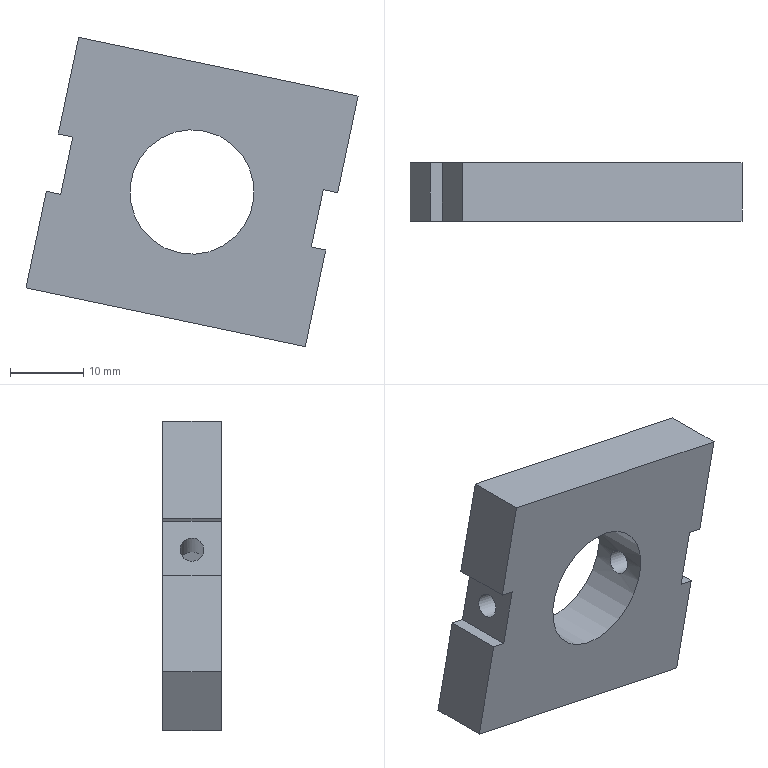Part | STEP file | SN10_006_002_PISADOR | 1 solid | 17 faces | box 45.364 x 8 x 42.272 mm | volume 8699 mm3 | plane 14 | cylinder 3 | commonest cylinder face diameters 3.242 x2 17 x1